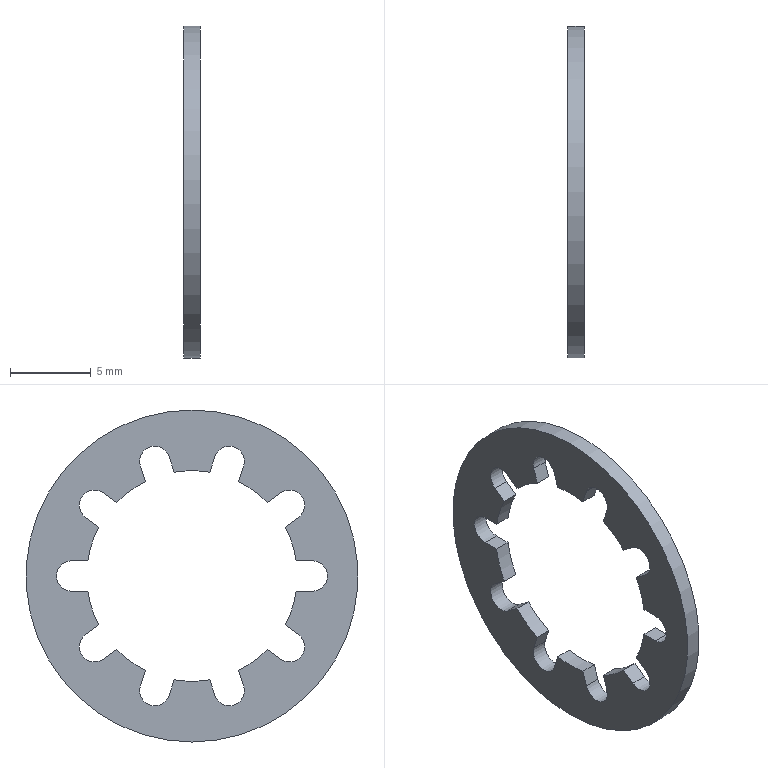Part | NX | features BREP 1 | 1 solid | 43 faces | box 1 x 20.5 x 20.5 mm | volume 165.523 mm3 | plane 22 | cylinder 21 | commonest cylinder face diameters 1.875 x10 13 x10 20.5 x1
STEP:
#1=CARTESIAN_POINT('',(0.,0.,10.25));
#2=VERTEX_POINT('',#1);
#3=CARTESIAN_POINT('',(0.,0.,0.));
#4=DIRECTION('',(1.,0.,0.));
#5=DIRECTION('',(0.,0.,1.));
#6=AXIS2_PLACEMENT_3D('',#3,#4,#5);
#7=CIRCLE('',#6,10.25);
#8=EDGE_CURVE('',#2,#2,#7,.T.);
#9=ORIENTED_EDGE('',*,*,#8,.F.);
#10=EDGE_LOOP('',(#9));
#11=FACE_BOUND('',#10,.T.);
#12=CARTESIAN_POINT('',(0.,3.19,6.784));
#13=VERTEX_POINT('',#12);
#14=CARTESIAN_POINT('',(0.,2.879,5.828));
#15=VERTEX_POINT('',#14);
#16=CARTESIAN_POINT('',(0.,3.19,6.784));
#17=DIRECTION('',(0.,-0.309,-0.9511));
#18=VECTOR('',#17,1000.);
#19=LINE('',#16,#18);
#20=EDGE_CURVE('',#13,#15,#19,.T.);
#21=ORIENTED_EDGE('',*,*,#20,.F.);
#22=CARTESIAN_POINT('',(0.,1.407,7.363));
#23=VERTEX_POINT('',#22);
#24=CARTESIAN_POINT('',(0.,2.298,7.073));
#25=DIRECTION('',(-1.,0.,0.));
#26=DIRECTION('',(0.,0.,1.));
#27=AXIS2_PLACEMENT_3D('',#24,#25,#26);
#28=CIRCLE('',#27,0.9375);
#29=EDGE_CURVE('',#23,#13,#28,.T.);
#30=ORIENTED_EDGE('',*,*,#29,.F.);
#31=CARTESIAN_POINT('',(0.,1.096,6.407));
#32=VERTEX_POINT('',#31);
#33=CARTESIAN_POINT('',(0.,1.096,6.407));
#34=DIRECTION('',(0.,0.309,0.9511));
#35=VECTOR('',#34,1000.);
#36=LINE('',#33,#35);
#37=EDGE_CURVE('',#32,#23,#36,.T.);
#38=ORIENTED_EDGE('',*,*,#37,.F.);
#39=CARTESIAN_POINT('',(0.,-1.096,6.407));
#40=VERTEX_POINT('',#39);
#41=CARTESIAN_POINT('',(0.,0.,0.));
#42=DIRECTION('',(-1.,0.,0.));
#43=DIRECTION('',(0.,0.,1.));
#44=AXIS2_PLACEMENT_3D('',#41,#42,#43);
#45=CIRCLE('',#44,6.5);
#46=EDGE_CURVE('',#40,#32,#45,.T.);
#47=ORIENTED_EDGE('',*,*,#46,.F.);
#48=CARTESIAN_POINT('',(0.,-1.407,7.363));
#49=VERTEX_POINT('',#48);
#50=CARTESIAN_POINT('',(0.,-1.407,7.363));
#51=DIRECTION('',(0.,0.309,-0.9511));
#52=VECTOR('',#51,1000.);
#53=LINE('',#50,#52);
#54=EDGE_CURVE('',#49,#40,#53,.T.);
#55=ORIENTED_EDGE('',*,*,#54,.F.);
#56=CARTESIAN_POINT('',(0.,-3.19,6.784));
#57=VERTEX_POINT('',#56);
#58=CARTESIAN_POINT('',(0.,-2.298,7.073));
#59=DIRECTION('',(-1.,0.,0.));
#60=DIRECTION('',(0.,0.,1.));
#61=AXIS2_PLACEMENT_3D('',#58,#59,#60);
#62=CIRCLE('',#61,0.9375);
#63=EDGE_CURVE('',#57,#49,#62,.T.);
#64=ORIENTED_EDGE('',*,*,#63,.F.);
#65=CARTESIAN_POINT('',(0.,-2.879,5.828));
#66=VERTEX_POINT('',#65);
#67=CARTESIAN_POINT('',(0.,-2.879,5.828));
#68=DIRECTION('',(0.,-0.309,0.9511));
#69=VECTOR('',#68,1000.);
#70=LINE('',#67,#69);
#71=EDGE_CURVE('',#66,#57,#70,.T.);
#72=ORIENTED_EDGE('',*,*,#71,.F.);
#73=CARTESIAN_POINT('',(0.,-4.653,4.539));
#74=VERTEX_POINT('',#73);
#75=CARTESIAN_POINT('',(0.,0.,0.));
#76=DIRECTION('',(-1.,0.,0.));
#77=DIRECTION('',(0.,0.,1.));
#78=AXIS2_PLACEMENT_3D('',#75,#76,#77);
#79=CIRCLE('',#78,6.5);
#80=EDGE_CURVE('',#74,#66,#79,.T.);
#81=ORIENTED_EDGE('',*,*,#80,.F.);
#82=CARTESIAN_POINT('',(0.,-5.466,5.13));
#83=VERTEX_POINT('',#82);
#84=CARTESIAN_POINT('',(0.,-5.466,5.13));
#85=DIRECTION('',(0.,0.809,-0.5878));
#86=VECTOR('',#85,1000.);
#87=LINE('',#84,#86);
#88=EDGE_CURVE('',#83,#74,#87,.T.);
#89=ORIENTED_EDGE('',*,*,#88,.F.);
#90=CARTESIAN_POINT('',(0.,-6.568,3.613));
#91=VERTEX_POINT('',#90);
#92=CARTESIAN_POINT('',(0.,-6.017,4.372));
#93=DIRECTION('',(-1.,0.,0.));
#94=DIRECTION('',(0.,0.,1.));
#95=AXIS2_PLACEMENT_3D('',#92,#93,#94);
#96=CIRCLE('',#95,0.9375);
#97=EDGE_CURVE('',#91,#83,#96,.T.);
#98=ORIENTED_EDGE('',*,*,#97,.F.);
#99=CARTESIAN_POINT('',(0.,-5.755,3.022));
#100=VERTEX_POINT('',#99);
#101=CARTESIAN_POINT('',(0.,-5.755,3.022));
#102=DIRECTION('',(0.,-0.809,0.5878));
#103=VECTOR('',#102,1000.);
#104=LINE('',#101,#103);
#105=EDGE_CURVE('',#100,#91,#104,.T.);
#106=ORIENTED_EDGE('',*,*,#105,.F.);
#107=CARTESIAN_POINT('',(0.,-6.432,0.9375));
#108=VERTEX_POINT('',#107);
#109=CARTESIAN_POINT('',(0.,0.,0.));
#110=DIRECTION('',(-1.,0.,0.));
#111=DIRECTION('',(0.,0.,1.));
#112=AXIS2_PLACEMENT_3D('',#109,#110,#111);
#113=CIRCLE('',#112,6.5);
#114=EDGE_CURVE('',#108,#100,#113,.T.);
#115=ORIENTED_EDGE('',*,*,#114,.F.);
#116=CARTESIAN_POINT('',(0.,-7.438,0.9375));
#117=VERTEX_POINT('',#116);
#118=CARTESIAN_POINT('',(0.,0.,0.9375));
#119=DIRECTION('',(0.,1.,0.));
#120=VECTOR('',#119,1000.);
#121=LINE('',#118,#120);
#122=EDGE_CURVE('',#117,#108,#121,.T.);
#123=ORIENTED_EDGE('',*,*,#122,.F.);
#124=CARTESIAN_POINT('',(0.,-7.438,-0.9375));
#125=VERTEX_POINT('',#124);
#126=CARTESIAN_POINT('',(0.,-7.438,0.));
#127=DIRECTION('',(-1.,0.,0.));
#128=DIRECTION('',(0.,0.,1.));
#129=AXIS2_PLACEMENT_3D('',#126,#127,#128);
#130=CIRCLE('',#129,0.9375);
#131=EDGE_CURVE('',#125,#117,#130,.T.);
#132=ORIENTED_EDGE('',*,*,#131,.F.);
#133=CARTESIAN_POINT('',(0.,-6.432,-0.9375));
#134=VERTEX_POINT('',#133);
#135=CARTESIAN_POINT('',(0.,0.,-0.9375));
#136=DIRECTION('',(0.,-1.,0.));
#137=VECTOR('',#136,1000.);
#138=LINE('',#135,#137);
#139=EDGE_CURVE('',#134,#125,#138,.T.);
#140=ORIENTED_EDGE('',*,*,#139,.F.);
#141=CARTESIAN_POINT('',(0.,-5.755,-3.022));
#142=VERTEX_POINT('',#141);
#143=CARTESIAN_POINT('',(0.,0.,0.));
#144=DIRECTION('',(-1.,0.,0.));
#145=DIRECTION('',(0.,0.,1.));
#146=AXIS2_PLACEMENT_3D('',#143,#144,#145);
#147=CIRCLE('',#146,6.5);
#148=EDGE_CURVE('',#142,#134,#147,.T.);
#149=ORIENTED_EDGE('',*,*,#148,.F.);
#150=CARTESIAN_POINT('',(0.,-6.568,-3.613));
#151=VERTEX_POINT('',#150);
#152=CARTESIAN_POINT('',(0.,-6.568,-3.613));
#153=DIRECTION('',(0.,0.809,0.5878));
#154=VECTOR('',#153,1000.);
#155=LINE('',#152,#154);
#156=EDGE_CURVE('',#151,#142,#155,.T.);
#157=ORIENTED_EDGE('',*,*,#156,.F.);
#158=CARTESIAN_POINT('',(0.,-5.466,-5.13));
#159=VERTEX_POINT('',#158);
#160=CARTESIAN_POINT('',(0.,-6.017,-4.372));
#161=DIRECTION('',(-1.,0.,0.));
#162=DIRECTION('',(0.,0.,1.));
#163=AXIS2_PLACEMENT_3D('',#160,#161,#162);
#164=CIRCLE('',#163,0.9375);
#165=EDGE_CURVE('',#159,#151,#164,.T.);
#166=ORIENTED_EDGE('',*,*,#165,.F.);
#167=CARTESIAN_POINT('',(0.,-4.653,-4.539));
#168=VERTEX_POINT('',#167);
#169=CARTESIAN_POINT('',(0.,-4.653,-4.539));
#170=DIRECTION('',(0.,-0.809,-0.5878));
#171=VECTOR('',#170,1000.);
#172=LINE('',#169,#171);
#173=EDGE_CURVE('',#168,#159,#172,.T.);
#174=ORIENTED_EDGE('',*,*,#173,.F.);
#175=CARTESIAN_POINT('',(0.,-2.879,-5.828));
#176=VERTEX_POINT('',#175);
#177=CARTESIAN_POINT('',(0.,0.,0.));
#178=DIRECTION('',(-1.,0.,0.));
#179=DIRECTION('',(0.,0.,1.));
#180=AXIS2_PLACEMENT_3D('',#177,#178,#179);
#181=CIRCLE('',#180,6.5);
#182=EDGE_CURVE('',#176,#168,#181,.T.);
#183=ORIENTED_EDGE('',*,*,#182,.F.);
#184=CARTESIAN_POINT('',(0.,-3.19,-6.784));
#185=VERTEX_POINT('',#184);
#186=CARTESIAN_POINT('',(0.,-3.19,-6.784));
#187=DIRECTION('',(0.,0.309,0.9511));
#188=VECTOR('',#187,1000.);
#189=LINE('',#186,#188);
#190=EDGE_CURVE('',#185,#176,#189,.T.);
#191=ORIENTED_EDGE('',*,*,#190,.F.);
#192=CARTESIAN_POINT('',(0.,-1.407,-7.363));
#193=VERTEX_POINT('',#192);
#194=CARTESIAN_POINT('',(0.,-2.298,-7.073));
#195=DIRECTION('',(-1.,0.,0.));
#196=DIRECTION('',(0.,0.,1.));
#197=AXIS2_PLACEMENT_3D('',#194,#195,#196);
#198=CIRCLE('',#197,0.9375);
#199=EDGE_CURVE('',#193,#185,#198,.T.);
#200=ORIENTED_EDGE('',*,*,#199,.F.);
#201=CARTESIAN_POINT('',(0.,-1.096,-6.407));
#202=VERTEX_POINT('',#201);
#203=CARTESIAN_POINT('',(0.,-1.096,-6.407));
#204=DIRECTION('',(0.,-0.309,-0.9511));
#205=VECTOR('',#204,1000.);
#206=LINE('',#203,#205);
#207=EDGE_CURVE('',#202,#193,#206,.T.);
#208=ORIENTED_EDGE('',*,*,#207,.F.);
#209=CARTESIAN_POINT('',(0.,1.096,-6.407));
#210=VERTEX_POINT('',#209);
#211=CARTESIAN_POINT('',(0.,0.,0.));
#212=DIRECTION('',(-1.,0.,0.));
#213=DIRECTION('',(0.,0.,1.));
#214=AXIS2_PLACEMENT_3D('',#211,#212,#213);
#215=CIRCLE('',#214,6.5);
#216=EDGE_CURVE('',#210,#202,#215,.T.);
#217=ORIENTED_EDGE('',*,*,#216,.F.);
#218=CARTESIAN_POINT('',(0.,1.407,-7.363));
#219=VERTEX_POINT('',#218);
#220=CARTESIAN_POINT('',(0.,1.407,-7.363));
#221=DIRECTION('',(0.,-0.309,0.9511));
#222=VECTOR('',#221,1000.);
#223=LINE('',#220,#222);
#224=EDGE_CURVE('',#219,#210,#223,.T.);
#225=ORIENTED_EDGE('',*,*,#224,.F.);
#226=CARTESIAN_POINT('',(0.,3.19,-6.784));
#227=VERTEX_POINT('',#226);
#228=CARTESIAN_POINT('',(0.,2.298,-7.073));
#229=DIRECTION('',(-1.,0.,0.));
#230=DIRECTION('',(0.,0.,1.));
#231=AXIS2_PLACEMENT_3D('',#228,#229,#230);
#232=CIRCLE('',#231,0.9375);
#233=EDGE_CURVE('',#227,#219,#232,.T.);
#234=ORIENTED_EDGE('',*,*,#233,.F.);
#235=CARTESIAN_POINT('',(0.,2.879,-5.828));
#236=VERTEX_POINT('',#235);
#237=CARTESIAN_POINT('',(0.,2.879,-5.828));
#238=DIRECTION('',(0.,0.309,-0.9511));
#239=VECTOR('',#238,1000.);
#240=LINE('',#237,#239);
#241=EDGE_CURVE('',#236,#227,#240,.T.);
#242=ORIENTED_EDGE('',*,*,#241,.F.);
#243=CARTESIAN_POINT('',(0.,4.653,-4.539));
#244=VERTEX_POINT('',#243);
#245=CARTESIAN_POINT('',(0.,0.,0.));
#246=DIRECTION('',(-1.,0.,0.));
#247=DIRECTION('',(0.,0.,1.));
#248=AXIS2_PLACEMENT_3D('',#245,#246,#247);
#249=CIRCLE('',#248,6.5);
#250=EDGE_CURVE('',#244,#236,#249,.T.);
#251=ORIENTED_EDGE('',*,*,#250,.F.);
#252=CARTESIAN_POINT('',(0.,5.466,-5.13));
#253=VERTEX_POINT('',#252);
#254=CARTESIAN_POINT('',(0.,5.466,-5.13));
#255=DIRECTION('',(0.,-0.809,0.5878));
#256=VECTOR('',#255,1000.);
#257=LINE('',#254,#256);
#258=EDGE_CURVE('',#253,#244,#257,.T.);
#259=ORIENTED_EDGE('',*,*,#258,.F.);
#260=CARTESIAN_POINT('',(0.,6.568,-3.613));
#261=VERTEX_POINT('',#260);
#262=CARTESIAN_POINT('',(0.,6.017,-4.372));
#263=DIRECTION('',(-1.,0.,0.));
#264=DIRECTION('',(0.,0.,1.));
#265=AXIS2_PLACEMENT_3D('',#262,#263,#264);
#266=CIRCLE('',#265,0.9375);
#267=EDGE_CURVE('',#261,#253,#266,.T.);
#268=ORIENTED_EDGE('',*,*,#267,.F.);
#269=CARTESIAN_POINT('',(0.,5.755,-3.022));
#270=VERTEX_POINT('',#269);
#271=CARTESIAN_POINT('',(0.,5.755,-3.022));
#272=DIRECTION('',(0.,0.809,-0.5878));
#273=VECTOR('',#272,1000.);
#274=LINE('',#271,#273);
#275=EDGE_CURVE('',#270,#261,#274,.T.);
#276=ORIENTED_EDGE('',*,*,#275,.F.);
#277=CARTESIAN_POINT('',(0.,6.432,-0.9375));
#278=VERTEX_POINT('',#277);
#279=CARTESIAN_POINT('',(0.,0.,0.));
#280=DIRECTION('',(-1.,0.,0.));
#281=DIRECTION('',(0.,0.,1.));
#282=AXIS2_PLACEMENT_3D('',#279,#280,#281);
#283=CIRCLE('',#282,6.5);
#284=EDGE_CURVE('',#278,#270,#283,.T.);
#285=ORIENTED_EDGE('',*,*,#284,.F.);
#286=CARTESIAN_POINT('',(0.,7.438,-0.9375));
#287=VERTEX_POINT('',#286);
#288=CARTESIAN_POINT('',(0.,0.,-0.9375));
#289=DIRECTION('',(0.,-1.,0.));
#290=VECTOR('',#289,1000.);
#291=LINE('',#288,#290);
#292=EDGE_CURVE('',#287,#278,#291,.T.);
#293=ORIENTED_EDGE('',*,*,#292,.F.);
#294=CARTESIAN_POINT('',(0.,7.438,0.9375));
#295=VERTEX_POINT('',#294);
#296=CARTESIAN_POINT('',(0.,7.438,0.));
#297=DIRECTION('',(-1.,0.,0.));
#298=DIRECTION('',(0.,0.,1.));
#299=AXIS2_PLACEMENT_3D('',#296,#297,#298);
#300=CIRCLE('',#299,0.9375);
#301=EDGE_CURVE('',#295,#287,#300,.T.);
#302=ORIENTED_EDGE('',*,*,#301,.F.);
#303=CARTESIAN_POINT('',(0.,6.432,0.9375));
#304=VERTEX_POINT('',#303);
#305=CARTESIAN_POINT('',(0.,0.,0.9375));
#306=DIRECTION('',(0.,1.,0.));
#307=VECTOR('',#306,1000.);
#308=LINE('',#305,#307);
#309=EDGE_CURVE('',#304,#295,#308,.T.);
#310=ORIENTED_EDGE('',*,*,#309,.F.);
#311=CARTESIAN_POINT('',(0.,5.755,3.022));
#312=VERTEX_POINT('',#311);
#313=CARTESIAN_POINT('',(0.,0.,0.));
#314=DIRECTION('',(-1.,0.,0.));
#315=DIRECTION('',(0.,0.,1.));
#316=AXIS2_PLACEMENT_3D('',#313,#314,#315);
#317=CIRCLE('',#316,6.5);
#318=EDGE_CURVE('',#312,#304,#317,.T.);
#319=ORIENTED_EDGE('',*,*,#318,.F.);
#320=CARTESIAN_POINT('',(0.,6.568,3.613));
#321=VERTEX_POINT('',#320);
#322=CARTESIAN_POINT('',(0.,6.568,3.613));
#323=DIRECTION('',(0.,-0.809,-0.5878));
#324=VECTOR('',#323,1000.);
#325=LINE('',#322,#324);
#326=EDGE_CURVE('',#321,#312,#325,.T.);
#327=ORIENTED_EDGE('',*,*,#326,.F.);
#328=CARTESIAN_POINT('',(0.,5.466,5.13));
#329=VERTEX_POINT('',#328);
#330=CARTESIAN_POINT('',(0.,6.017,4.372));
#331=DIRECTION('',(-1.,0.,0.));
#332=DIRECTION('',(0.,0.,1.));
#333=AXIS2_PLACEMENT_3D('',#330,#331,#332);
#334=CIRCLE('',#333,0.9375);
#335=EDGE_CURVE('',#329,#321,#334,.T.);
#336=ORIENTED_EDGE('',*,*,#335,.F.);
#337=CARTESIAN_POINT('',(0.,4.653,4.539));
#338=VERTEX_POINT('',#337);
#339=CARTESIAN_POINT('',(0.,4.653,4.539));
#340=DIRECTION('',(0.,0.809,0.5878));
#341=VECTOR('',#340,1000.);
#342=LINE('',#339,#341);
#343=EDGE_CURVE('',#338,#329,#342,.T.);
#344=ORIENTED_EDGE('',*,*,#343,.F.);
#345=CARTESIAN_POINT('',(0.,0.,0.));
#346=DIRECTION('',(-1.,0.,0.));
#347=DIRECTION('',(0.,0.,1.));
#348=AXIS2_PLACEMENT_3D('',#345,#346,#347);
#349=CIRCLE('',#348,6.5);
#350=EDGE_CURVE('',#15,#338,#349,.T.);
#351=ORIENTED_EDGE('',*,*,#350,.F.);
#352=EDGE_LOOP('',(#21,#30,#38,#47,#55,#64,#72,#81,#89,#98,#106,#115,#123,#132,#140,#149,#157,#166,#174,#183,#191,#200,#208,#217,#225,#234,#242,#251,#259,#268,#276,#285,#293,#302,#310,#319,#327,#336,#344,#351));
#353=FACE_BOUND('',#352,.T.);
#354=CARTESIAN_POINT('',(0.,0.,0.));
#355=DIRECTION('',(1.,0.,0.));
#356=DIRECTION('',(0.,0.,1.));
#357=AXIS2_PLACEMENT_3D('',#354,#355,#356);
#358=PLANE('',#357);
#359=ADVANCED_FACE('',(#11,#353),#358,.F.);
#360=CARTESIAN_POINT('',(1.,0.,10.25));
#361=VERTEX_POINT('',#360);
#362=CARTESIAN_POINT('',(1.,0.,0.));
#363=DIRECTION('',(-1.,0.,0.));
#364=DIRECTION('',(0.,0.,1.));
#365=AXIS2_PLACEMENT_3D('',#362,#363,#364);
#366=CIRCLE('',#365,10.25);
#367=EDGE_CURVE('',#361,#361,#366,.T.);
#368=ORIENTED_EDGE('',*,*,#367,.T.);
#369=EDGE_LOOP('',(#368));
#370=FACE_BOUND('',#369,.T.);
#371=ORIENTED_EDGE('',*,*,#8,.T.);
#372=EDGE_LOOP('',(#371));
#373=FACE_BOUND('',#372,.T.);
#374=CARTESIAN_POINT('',(1.,0.,0.));
#375=DIRECTION('',(-1.,0.,0.));
#376=DIRECTION('',(0.,0.,-1.));
#377=AXIS2_PLACEMENT_3D('',#374,#375,#376);
#378=CYLINDRICAL_SURFACE('',#377,10.25);
#379=ADVANCED_FACE('',(#370,#373),#378,.T.);
#380=CARTESIAN_POINT('',(1.,2.879,5.828));
#381=VERTEX_POINT('',#380);
#382=CARTESIAN_POINT('',(1.,3.19,6.784));
#383=VERTEX_POINT('',#382);
#384=CARTESIAN_POINT('',(1.,2.879,5.828));
#385=DIRECTION('',(0.,0.309,0.9511));
#386=VECTOR('',#385,1000.);
#387=LINE('',#384,#386);
#388=EDGE_CURVE('',#381,#383,#387,.T.);
#389=ORIENTED_EDGE('',*,*,#388,.T.);
#390=CARTESIAN_POINT('',(1.,3.19,6.784));
#391=DIRECTION('',(-1.,0.,0.));
#392=VECTOR('',#391,1000.);
#393=LINE('',#390,#392);
#394=EDGE_CURVE('',#383,#13,#393,.T.);
#395=ORIENTED_EDGE('',*,*,#394,.T.);
#396=ORIENTED_EDGE('',*,*,#20,.T.);
#397=CARTESIAN_POINT('',(1.,2.879,5.828));
#398=DIRECTION('',(1.,0.,0.));
#399=VECTOR('',#398,1000.);
#400=LINE('',#397,#399);
#401=EDGE_CURVE('',#15,#381,#400,.T.);
#402=ORIENTED_EDGE('',*,*,#401,.T.);
#403=EDGE_LOOP('',(#389,#395,#396,#402));
#404=FACE_BOUND('',#403,.T.);
#405=CARTESIAN_POINT('',(1.,2.879,5.828));
#406=DIRECTION('',(0.,-0.9511,0.309));
#407=DIRECTION('',(0.,0.309,0.9511));
#408=AXIS2_PLACEMENT_3D('',#405,#406,#407);
#409=PLANE('',#408);
#410=ADVANCED_FACE('',(#404),#409,.T.);
#411=CARTESIAN_POINT('',(1.,1.407,7.363));
#412=VERTEX_POINT('',#411);
#413=CARTESIAN_POINT('',(1.,2.298,7.073));
#414=DIRECTION('',(-1.,0.,0.));
#415=DIRECTION('',(0.,0.,1.));
#416=AXIS2_PLACEMENT_3D('',#413,#414,#415);
#417=CIRCLE('',#416,0.9375);
#418=EDGE_CURVE('',#412,#383,#417,.T.);
#419=ORIENTED_EDGE('',*,*,#418,.F.);
#420=CARTESIAN_POINT('',(1.,1.407,7.363));
#421=DIRECTION('',(1.,0.,0.));
#422=VECTOR('',#421,1000.);
#423=LINE('',#420,#422);
#424=EDGE_CURVE('',#23,#412,#423,.T.);
#425=ORIENTED_EDGE('',*,*,#424,.F.);
#426=ORIENTED_EDGE('',*,*,#29,.T.);
#427=ORIENTED_EDGE('',*,*,#394,.F.);
#428=EDGE_LOOP('',(#419,#425,#426,#427));
#429=FACE_BOUND('',#428,.T.);
#430=CARTESIAN_POINT('',(1.,2.298,7.073));
#431=DIRECTION('',(-1.,0.,0.));
#432=DIRECTION('',(0.,0.,-1.));
#433=AXIS2_PLACEMENT_3D('',#430,#431,#432);
#434=CYLINDRICAL_SURFACE('',#433,0.9375);
#435=ADVANCED_FACE('',(#429),#434,.F.);
#436=CARTESIAN_POINT('',(1.,1.096,6.407));
#437=VERTEX_POINT('',#436);
#438=CARTESIAN_POINT('',(1.,1.407,7.363));
#439=DIRECTION('',(0.,-0.309,-0.9511));
#440=VECTOR('',#439,1000.);
#441=LINE('',#438,#440);
#442=EDGE_CURVE('',#412,#437,#441,.T.);
#443=ORIENTED_EDGE('',*,*,#442,.T.);
#444=CARTESIAN_POINT('',(1.,1.096,6.407));
#445=DIRECTION('',(-1.,0.,0.));
#446=VECTOR('',#445,1000.);
#447=LINE('',#444,#446);
#448=EDGE_CURVE('',#437,#32,#447,.T.);
#449=ORIENTED_EDGE('',*,*,#448,.T.);
#450=ORIENTED_EDGE('',*,*,#37,.T.);
#451=ORIENTED_EDGE('',*,*,#424,.T.);
#452=EDGE_LOOP('',(#443,#449,#450,#451));
#453=FACE_BOUND('',#452,.T.);
#454=CARTESIAN_POINT('',(1.,1.407,7.363));
#455=DIRECTION('',(0.,0.9511,-0.309));
#456=DIRECTION('',(0.,-0.309,-0.9511));
#457=AXIS2_PLACEMENT_3D('',#454,#455,#456);
#458=PLANE('',#457);
#459=ADVANCED_FACE('',(#453),#458,.T.);
#460=CARTESIAN_POINT('',(1.,-1.096,6.407));
#461=VERTEX_POINT('',#460);
#462=CARTESIAN_POINT('',(1.,0.,0.));
#463=DIRECTION('',(-1.,0.,0.));
#464=DIRECTION('',(0.,0.,1.));
#465=AXIS2_PLACEMENT_3D('',#462,#463,#464);
#466=CIRCLE('',#465,6.5);
#467=EDGE_CURVE('',#461,#437,#466,.T.);
#468=ORIENTED_EDGE('',*,*,#467,.F.);
#469=CARTESIAN_POINT('',(1.,-1.096,6.407));
#470=DIRECTION('',(1.,0.,0.));
#471=VECTOR('',#470,1000.);
#472=LINE('',#469,#471);
#473=EDGE_CURVE('',#40,#461,#472,.T.);
#474=ORIENTED_EDGE('',*,*,#473,.F.);
#475=ORIENTED_EDGE('',*,*,#46,.T.);
#476=ORIENTED_EDGE('',*,*,#448,.F.);
#477=EDGE_LOOP('',(#468,#474,#475,#476));
#478=FACE_BOUND('',#477,.T.);
#479=CARTESIAN_POINT('',(1.,0.,0.));
#480=DIRECTION('',(-1.,0.,0.));
#481=DIRECTION('',(0.,0.,-1.));
#482=AXIS2_PLACEMENT_3D('',#479,#480,#481);
#483=CYLINDRICAL_SURFACE('',#482,6.5);
#484=ADVANCED_FACE('',(#478),#483,.F.);
#485=CARTESIAN_POINT('',(1.,-1.407,7.363));
#486=VERTEX_POINT('',#485);
#487=CARTESIAN_POINT('',(1.,-1.096,6.407));
#488=DIRECTION('',(0.,-0.309,0.9511));
#489=VECTOR('',#488,1000.);
#490=LINE('',#487,#489);
#491=EDGE_CURVE('',#461,#486,#490,.T.);
#492=ORIENTED_EDGE('',*,*,#491,.T.);
#493=CARTESIAN_POINT('',(1.,-1.407,7.363));
#494=DIRECTION('',(-1.,0.,0.));
#495=VECTOR('',#494,1000.);
#496=LINE('',#493,#495);
#497=EDGE_CURVE('',#486,#49,#496,.T.);
#498=ORIENTED_EDGE('',*,*,#497,.T.);
#499=ORIENTED_EDGE('',*,*,#54,.T.);
#500=ORIENTED_EDGE('',*,*,#473,.T.);
#501=EDGE_LOOP('',(#492,#498,#499,#500));
#502=FACE_BOUND('',#501,.T.);
#503=CARTESIAN_POINT('',(1.,-1.096,6.407));
#504=DIRECTION('',(0.,-0.9511,-0.309));
#505=DIRECTION('',(0.,-0.309,0.9511));
#506=AXIS2_PLACEMENT_3D('',#503,#504,#505);
#507=PLANE('',#506);
#508=ADVANCED_FACE('',(#502),#507,.T.);
#509=CARTESIAN_POINT('',(1.,-3.19,6.784));
#510=VERTEX_POINT('',#509);
#511=CARTESIAN_POINT('',(1.,-2.298,7.073));
#512=DIRECTION('',(-1.,0.,0.));
#513=DIRECTION('',(0.,0.,1.));
#514=AXIS2_PLACEMENT_3D('',#511,#512,#513);
#515=CIRCLE('',#514,0.9375);
#516=EDGE_CURVE('',#510,#486,#515,.T.);
#517=ORIENTED_EDGE('',*,*,#516,.F.);
#518=CARTESIAN_POINT('',(1.,-3.19,6.784));
#519=DIRECTION('',(1.,0.,0.));
#520=VECTOR('',#519,1000.);
#521=LINE('',#518,#520);
#522=EDGE_CURVE('',#57,#510,#521,.T.);
#523=ORIENTED_EDGE('',*,*,#522,.F.);
#524=ORIENTED_EDGE('',*,*,#63,.T.);
#525=ORIENTED_EDGE('',*,*,#497,.F.);
#526=EDGE_LOOP('',(#517,#523,#524,#525));
#527=FACE_BOUND('',#526,.T.);
#528=CARTESIAN_POINT('',(1.,-2.298,7.073));
#529=DIRECTION('',(-1.,0.,0.));
#530=DIRECTION('',(0.,0.,-1.));
#531=AXIS2_PLACEMENT_3D('',#528,#529,#530);
#532=CYLINDRICAL_SURFACE('',#531,0.9375);
#533=ADVANCED_FACE('',(#527),#532,.F.);
#534=CARTESIAN_POINT('',(1.,-2.879,5.828));
#535=VERTEX_POINT('',#534);
#536=CARTESIAN_POINT('',(1.,-3.19,6.784));
#537=DIRECTION('',(0.,0.309,-0.9511));
#538=VECTOR('',#537,1000.);
#539=LINE('',#536,#538);
#540=EDGE_CURVE('',#510,#535,#539,.T.);
#541=ORIENTED_EDGE('',*,*,#540,.T.);
#542=CARTESIAN_POINT('',(1.,-2.879,5.828));
#543=DIRECTION('',(-1.,0.,0.));
#544=VECTOR('',#543,1000.);
#545=LINE('',#542,#544);
#546=EDGE_CURVE('',#535,#66,#545,.T.);
#547=ORIENTED_EDGE('',*,*,#546,.T.);
#548=ORIENTED_EDGE('',*,*,#71,.T.);
#549=ORIENTED_EDGE('',*,*,#522,.T.);
#550=EDGE_LOOP('',(#541,#547,#548,#549));
#551=FACE_BOUND('',#550,.T.);
#552=CARTESIAN_POINT('',(1.,-3.19,6.784));
#553=DIRECTION('',(0.,0.9511,0.309));
#554=DIRECTION('',(0.,0.309,-0.9511));
#555=AXIS2_PLACEMENT_3D('',#552,#553,#554);
#556=PLANE('',#555);
#557=ADVANCED_FACE('',(#551),#556,.T.);
#558=ORIENTED_EDGE('',*,*,#546,.F.);
#559=CARTESIAN_POINT('',(1.,-4.653,4.539));
#560=VERTEX_POINT('',#559);
#561=CARTESIAN_POINT('',(1.,0.,0.));
#562=DIRECTION('',(-1.,0.,0.));
#563=DIRECTION('',(0.,0.,1.));
#564=AXIS2_PLACEMENT_3D('',#561,#562,#563);
#565=CIRCLE('',#564,6.5);
#566=EDGE_CURVE('',#560,#535,#565,.T.);
#567=ORIENTED_EDGE('',*,*,#566,.F.);
#568=CARTESIAN_POINT('',(1.,-4.653,4.539));
#569=DIRECTION('',(1.,0.,0.));
#570=VECTOR('',#569,1000.);
#571=LINE('',#568,#570);
#572=EDGE_CURVE('',#74,#560,#571,.T.);
#573=ORIENTED_EDGE('',*,*,#572,.F.);
#574=ORIENTED_EDGE('',*,*,#80,.T.);
#575=EDGE_LOOP('',(#558,#567,#573,#574));
#576=FACE_BOUND('',#575,.T.);
#577=CARTESIAN_POINT('',(1.,0.,0.));
#578=DIRECTION('',(-1.,0.,0.));
#579=DIRECTION('',(0.,0.,-1.));
#580=AXIS2_PLACEMENT_3D('',#577,#578,#579);
#581=CYLINDRICAL_SURFACE('',#580,6.5);
#582=ADVANCED_FACE('',(#576),#581,.F.);
#583=CARTESIAN_POINT('',(1.,-5.466,5.13));
#584=VERTEX_POINT('',#583);
#585=CARTESIAN_POINT('',(1.,-4.653,4.539));
#586=DIRECTION('',(0.,-0.809,0.5878));
#587=VECTOR('',#586,1000.);
#588=LINE('',#585,#587);
#589=EDGE_CURVE('',#560,#584,#588,.T.);
#590=ORIENTED_EDGE('',*,*,#589,.T.);
#591=CARTESIAN_POINT('',(1.,-5.466,5.13));
#592=DIRECTION('',(-1.,0.,0.));
#593=VECTOR('',#592,1000.);
#594=LINE('',#591,#593);
#595=EDGE_CURVE('',#584,#83,#594,.T.);
#596=ORIENTED_EDGE('',*,*,#595,.T.);
#597=ORIENTED_EDGE('',*,*,#88,.T.);
#598=ORIENTED_EDGE('',*,*,#572,.T.);
#599=EDGE_LOOP('',(#590,#596,#597,#598));
#600=FACE_BOUND('',#599,.T.);
#601=CARTESIAN_POINT('',(1.,-4.653,4.539));
#602=DIRECTION('',(0.,-0.5878,-0.809));
#603=DIRECTION('',(0.,-0.809,0.5878));
#604=AXIS2_PLACEMENT_3D('',#601,#602,#603);
#605=PLANE('',#604);
#606=ADVANCED_FACE('',(#600),#605,.T.);
#607=CARTESIAN_POINT('',(1.,-6.568,3.613));
#608=VERTEX_POINT('',#607);
#609=CARTESIAN_POINT('',(1.,-6.017,4.372));
#610=DIRECTION('',(-1.,0.,0.));
#611=DIRECTION('',(0.,0.,1.));
#612=AXIS2_PLACEMENT_3D('',#609,#610,#611);
#613=CIRCLE('',#612,0.9375);
#614=EDGE_CURVE('',#608,#584,#613,.T.);
#615=ORIENTED_EDGE('',*,*,#614,.F.);
#616=CARTESIAN_POINT('',(1.,-6.568,3.613));
#617=DIRECTION('',(1.,0.,0.));
#618=VECTOR('',#617,1000.);
#619=LINE('',#616,#618);
#620=EDGE_CURVE('',#91,#608,#619,.T.);
#621=ORIENTED_EDGE('',*,*,#620,.F.);
#622=ORIENTED_EDGE('',*,*,#97,.T.);
#623=ORIENTED_EDGE('',*,*,#595,.F.);
#624=EDGE_LOOP('',(#615,#621,#622,#623));
#625=FACE_BOUND('',#624,.T.);
#626=CARTESIAN_POINT('',(1.,-6.017,4.372));
#627=DIRECTION('',(-1.,0.,0.));
#628=DIRECTION('',(0.,0.,-1.));
#629=AXIS2_PLACEMENT_3D('',#626,#627,#628);
#630=CYLINDRICAL_SURFACE('',#629,0.9375);
#631=ADVANCED_FACE('',(#625),#630,.F.);
#632=CARTESIAN_POINT('',(1.,-5.755,3.022));
#633=VERTEX_POINT('',#632);
#634=CARTESIAN_POINT('',(1.,-6.568,3.613));
#635=DIRECTION('',(0.,0.809,-0.5878));
#636=VECTOR('',#635,1000.);
#637=LINE('',#634,#636);
#638=EDGE_CURVE('',#608,#633,#637,.T.);
#639=ORIENTED_EDGE('',*,*,#638,.T.);
#640=CARTESIAN_POINT('',(1.,-5.755,3.022));
#641=DIRECTION('',(-1.,0.,0.));
#642=VECTOR('',#641,1000.);
#643=LINE('',#640,#642);
#644=EDGE_CURVE('',#633,#100,#643,.T.);
#645=ORIENTED_EDGE('',*,*,#644,.T.);
#646=ORIENTED_EDGE('',*,*,#105,.T.);
#647=ORIENTED_EDGE('',*,*,#620,.T.);
#648=EDGE_LOOP('',(#639,#645,#646,#647));
#649=FACE_BOUND('',#648,.T.);
#650=CARTESIAN_POINT('',(1.,-6.568,3.613));
#651=DIRECTION('',(0.,0.5878,0.809));
#652=DIRECTION('',(0.,0.809,-0.5878));
#653=AXIS2_PLACEMENT_3D('',#650,#651,#652);
#654=PLANE('',#653);
#655=ADVANCED_FACE('',(#649),#654,.T.);
#656=ORIENTED_EDGE('',*,*,#644,.F.);
#657=CARTESIAN_POINT('',(1.,-6.432,0.9375));
#658=VERTEX_POINT('',#657);
#659=CARTESIAN_POINT('',(1.,0.,0.));
#660=DIRECTION('',(-1.,0.,0.));
#661=DIRECTION('',(0.,0.,1.));
#662=AXIS2_PLACEMENT_3D('',#659,#660,#661);
#663=CIRCLE('',#662,6.5);
#664=EDGE_CURVE('',#658,#633,#663,.T.);
#665=ORIENTED_EDGE('',*,*,#664,.F.);
#666=CARTESIAN_POINT('',(1.,-6.432,0.9375));
#667=DIRECTION('',(1.,0.,0.));
#668=VECTOR('',#667,1000.);
#669=LINE('',#666,#668);
#670=EDGE_CURVE('',#108,#658,#669,.T.);
#671=ORIENTED_EDGE('',*,*,#670,.F.);
#672=ORIENTED_EDGE('',*,*,#114,.T.);
#673=EDGE_LOOP('',(#656,#665,#671,#672));
#674=FACE_BOUND('',#673,.T.);
#675=CARTESIAN_POINT('',(1.,0.,0.));
#676=DIRECTION('',(-1.,0.,0.));
#677=DIRECTION('',(0.,0.,-1.));
#678=AXIS2_PLACEMENT_3D('',#675,#676,#677);
#679=CYLINDRICAL_SURFACE('',#678,6.5);
#680=ADVANCED_FACE('',(#674),#679,.F.);
#681=CARTESIAN_POINT('',(1.,-7.438,0.9375));
#682=VERTEX_POINT('',#681);
#683=CARTESIAN_POINT('',(1.,-6.432,0.9375));
#684=DIRECTION('',(0.,-1.,0.));
#685=VECTOR('',#684,1000.);
#686=LINE('',#683,#685);
#687=EDGE_CURVE('',#658,#682,#686,.T.);
#688=ORIENTED_EDGE('',*,*,#687,.T.);
#689=CARTESIAN_POINT('',(1.,-7.438,0.9375));
#690=DIRECTION('',(-1.,0.,0.));
#691=VECTOR('',#690,1000.);
#692=LINE('',#689,#691);
#693=EDGE_CURVE('',#682,#117,#692,.T.);
#694=ORIENTED_EDGE('',*,*,#693,.T.);
#695=ORIENTED_EDGE('',*,*,#122,.T.);
#696=ORIENTED_EDGE('',*,*,#670,.T.);
#697=EDGE_LOOP('',(#688,#694,#695,#696));
#698=FACE_BOUND('',#697,.T.);
#699=CARTESIAN_POINT('',(1.,-6.432,0.9375));
#700=DIRECTION('',(0.,0.,-1.));
#701=DIRECTION('',(1.,0.,0.));
#702=AXIS2_PLACEMENT_3D('',#699,#700,#701);
#703=PLANE('',#702);
#704=ADVANCED_FACE('',(#698),#703,.T.);
#705=ORIENTED_EDGE('',*,*,#693,.F.);
#706=CARTESIAN_POINT('',(1.,-7.438,-0.9375));
#707=VERTEX_POINT('',#706);
#708=CARTESIAN_POINT('',(1.,-7.438,0.));
#709=DIRECTION('',(-1.,0.,0.));
#710=DIRECTION('',(0.,0.,1.));
#711=AXIS2_PLACEMENT_3D('',#708,#709,#710);
#712=CIRCLE('',#711,0.9375);
#713=EDGE_CURVE('',#707,#682,#712,.T.);
#714=ORIENTED_EDGE('',*,*,#713,.F.);
#715=CARTESIAN_POINT('',(1.,-7.438,-0.9375));
#716=DIRECTION('',(1.,0.,0.));
#717=VECTOR('',#716,1000.);
#718=LINE('',#715,#717);
#719=EDGE_CURVE('',#125,#707,#718,.T.);
#720=ORIENTED_EDGE('',*,*,#719,.F.);
#721=ORIENTED_EDGE('',*,*,#131,.T.);
#722=EDGE_LOOP('',(#705,#714,#720,#721));
#723=FACE_BOUND('',#722,.T.);
#724=CARTESIAN_POINT('',(1.,-7.438,0.));
#725=DIRECTION('',(-1.,0.,0.));
#726=DIRECTION('',(0.,0.,-1.));
#727=AXIS2_PLACEMENT_3D('',#724,#725,#726);
#728=CYLINDRICAL_SURFACE('',#727,0.9375);
#729=ADVANCED_FACE('',(#723),#728,.F.);
#730=CARTESIAN_POINT('',(1.,-6.432,-0.9375));
#731=VERTEX_POINT('',#730);
#732=CARTESIAN_POINT('',(1.,-7.438,-0.9375));
#733=DIRECTION('',(0.,1.,0.));
#734=VECTOR('',#733,1000.);
#735=LINE('',#732,#734);
#736=EDGE_CURVE('',#707,#731,#735,.T.);
#737=ORIENTED_EDGE('',*,*,#736,.T.);
#738=CARTESIAN_POINT('',(1.,-6.432,-0.9375));
#739=DIRECTION('',(-1.,0.,0.));
#740=VECTOR('',#739,1000.);
#741=LINE('',#738,#740);
#742=EDGE_CURVE('',#731,#134,#741,.T.);
#743=ORIENTED_EDGE('',*,*,#742,.T.);
#744=ORIENTED_EDGE('',*,*,#139,.T.);
#745=ORIENTED_EDGE('',*,*,#719,.T.);
#746=EDGE_LOOP('',(#737,#743,#744,#745));
#747=FACE_BOUND('',#746,.T.);
#748=CARTESIAN_POINT('',(1.,-7.438,-0.9375));
#749=DIRECTION('',(0.,0.,1.));
#750=DIRECTION('',(0.,1.,0.));
#751=AXIS2_PLACEMENT_3D('',#748,#749,#750);
#752=PLANE('',#751);
#753=ADVANCED_FACE('',(#747),#752,.T.);
#754=ORIENTED_EDGE('',*,*,#742,.F.);
#755=CARTESIAN_POINT('',(1.,-5.755,-3.022));
#756=VERTEX_POINT('',#755);
#757=CARTESIAN_POINT('',(1.,0.,0.));
#758=DIRECTION('',(-1.,0.,0.));
#759=DIRECTION('',(0.,0.,1.));
#760=AXIS2_PLACEMENT_3D('',#757,#758,#759);
#761=CIRCLE('',#760,6.5);
#762=EDGE_CURVE('',#756,#731,#761,.T.);
#763=ORIENTED_EDGE('',*,*,#762,.F.);
#764=CARTESIAN_POINT('',(1.,-5.755,-3.022));
#765=DIRECTION('',(1.,0.,0.));
#766=VECTOR('',#765,1000.);
#767=LINE('',#764,#766);
#768=EDGE_CURVE('',#142,#756,#767,.T.);
#769=ORIENTED_EDGE('',*,*,#768,.F.);
#770=ORIENTED_EDGE('',*,*,#148,.T.);
#771=EDGE_LOOP('',(#754,#763,#769,#770));
#772=FACE_BOUND('',#771,.T.);
#773=CARTESIAN_POINT('',(1.,0.,0.));
#774=DIRECTION('',(-1.,0.,0.));
#775=DIRECTION('',(0.,0.,-1.));
#776=AXIS2_PLACEMENT_3D('',#773,#774,#775);
#777=CYLINDRICAL_SURFACE('',#776,6.5);
#778=ADVANCED_FACE('',(#772),#777,.F.);
#779=CARTESIAN_POINT('',(1.,-6.568,-3.613));
#780=VERTEX_POINT('',#779);
#781=CARTESIAN_POINT('',(1.,-5.755,-3.022));
#782=DIRECTION('',(0.,-0.809,-0.5878));
#783=VECTOR('',#782,1000.);
#784=LINE('',#781,#783);
#785=EDGE_CURVE('',#756,#780,#784,.T.);
#786=ORIENTED_EDGE('',*,*,#785,.T.);
#787=CARTESIAN_POINT('',(1.,-6.568,-3.613));
#788=DIRECTION('',(-1.,0.,0.));
#789=VECTOR('',#788,1000.);
#790=LINE('',#787,#789);
#791=EDGE_CURVE('',#780,#151,#790,.T.);
#792=ORIENTED_EDGE('',*,*,#791,.T.);
#793=ORIENTED_EDGE('',*,*,#156,.T.);
#794=ORIENTED_EDGE('',*,*,#768,.T.);
#795=EDGE_LOOP('',(#786,#792,#793,#794));
#796=FACE_BOUND('',#795,.T.);
#797=CARTESIAN_POINT('',(1.,-5.755,-3.022));
#798=DIRECTION('',(0.,0.5878,-0.809));
#799=DIRECTION('',(0.,-0.809,-0.5878));
#800=AXIS2_PLACEMENT_3D('',#797,#798,#799);
#801=PLANE('',#800);
#802=ADVANCED_FACE('',(#796),#801,.T.);
#803=ORIENTED_EDGE('',*,*,#791,.F.);
#804=CARTESIAN_POINT('',(1.,-5.466,-5.13));
#805=VERTEX_POINT('',#804);
#806=CARTESIAN_POINT('',(1.,-6.017,-4.372));
#807=DIRECTION('',(-1.,0.,0.));
#808=DIRECTION('',(0.,0.,1.));
#809=AXIS2_PLACEMENT_3D('',#806,#807,#808);
#810=CIRCLE('',#809,0.9375);
#811=EDGE_CURVE('',#805,#780,#810,.T.);
#812=ORIENTED_EDGE('',*,*,#811,.F.);
#813=CARTESIAN_POINT('',(1.,-5.466,-5.13));
#814=DIRECTION('',(1.,0.,0.));
#815=VECTOR('',#814,1000.);
#816=LINE('',#813,#815);
#817=EDGE_CURVE('',#159,#805,#816,.T.);
#818=ORIENTED_EDGE('',*,*,#817,.F.);
#819=ORIENTED_EDGE('',*,*,#165,.T.);
#820=EDGE_LOOP('',(#803,#812,#818,#819));
#821=FACE_BOUND('',#820,.T.);
#822=CARTESIAN_POINT('',(1.,-6.017,-4.372));
#823=DIRECTION('',(-1.,0.,0.));
#824=DIRECTION('',(0.,0.,-1.));
#825=AXIS2_PLACEMENT_3D('',#822,#823,#824);
#826=CYLINDRICAL_SURFACE('',#825,0.9375);
#827=ADVANCED_FACE('',(#821),#826,.F.);
#828=CARTESIAN_POINT('',(1.,-4.653,-4.539));
#829=VERTEX_POINT('',#828);
#830=CARTESIAN_POINT('',(1.,-5.466,-5.13));
#831=DIRECTION('',(0.,0.809,0.5878));
#832=VECTOR('',#831,1000.);
#833=LINE('',#830,#832);
#834=EDGE_CURVE('',#805,#829,#833,.T.);
#835=ORIENTED_EDGE('',*,*,#834,.T.);
#836=CARTESIAN_POINT('',(1.,-4.653,-4.539));
#837=DIRECTION('',(-1.,0.,0.));
#838=VECTOR('',#837,1000.);
#839=LINE('',#836,#838);
#840=EDGE_CURVE('',#829,#168,#839,.T.);
#841=ORIENTED_EDGE('',*,*,#840,.T.);
#842=ORIENTED_EDGE('',*,*,#173,.T.);
#843=ORIENTED_EDGE('',*,*,#817,.T.);
#844=EDGE_LOOP('',(#835,#841,#842,#843));
#845=FACE_BOUND('',#844,.T.);
#846=CARTESIAN_POINT('',(1.,-5.466,-5.13));
#847=DIRECTION('',(0.,-0.5878,0.809));
#848=DIRECTION('',(0.,0.809,0.5878));
#849=AXIS2_PLACEMENT_3D('',#846,#847,#848);
#850=PLANE('',#849);
#851=ADVANCED_FACE('',(#845),#850,.T.);
#852=ORIENTED_EDGE('',*,*,#840,.F.);
#853=CARTESIAN_POINT('',(1.,-2.879,-5.828));
#854=VERTEX_POINT('',#853);
#855=CARTESIAN_POINT('',(1.,0.,0.));
#856=DIRECTION('',(-1.,0.,0.));
#857=DIRECTION('',(0.,0.,1.));
#858=AXIS2_PLACEMENT_3D('',#855,#856,#857);
#859=CIRCLE('',#858,6.5);
#860=EDGE_CURVE('',#854,#829,#859,.T.);
#861=ORIENTED_EDGE('',*,*,#860,.F.);
#862=CARTESIAN_POINT('',(1.,-2.879,-5.828));
#863=DIRECTION('',(1.,0.,0.));
#864=VECTOR('',#863,1000.);
#865=LINE('',#862,#864);
#866=EDGE_CURVE('',#176,#854,#865,.T.);
#867=ORIENTED_EDGE('',*,*,#866,.F.);
#868=ORIENTED_EDGE('',*,*,#182,.T.);
#869=EDGE_LOOP('',(#852,#861,#867,#868));
#870=FACE_BOUND('',#869,.T.);
#871=CARTESIAN_POINT('',(1.,0.,0.));
#872=DIRECTION('',(-1.,0.,0.));
#873=DIRECTION('',(0.,0.,-1.));
#874=AXIS2_PLACEMENT_3D('',#871,#872,#873);
#875=CYLINDRICAL_SURFACE('',#874,6.5);
#876=ADVANCED_FACE('',(#870),#875,.F.);
#877=CARTESIAN_POINT('',(1.,-3.19,-6.784));
#878=VERTEX_POINT('',#877);
#879=CARTESIAN_POINT('',(1.,-2.879,-5.828));
#880=DIRECTION('',(0.,-0.309,-0.9511));
#881=VECTOR('',#880,1000.);
#882=LINE('',#879,#881);
#883=EDGE_CURVE('',#854,#878,#882,.T.);
#884=ORIENTED_EDGE('',*,*,#883,.T.);
#885=CARTESIAN_POINT('',(1.,-3.19,-6.784));
#886=DIRECTION('',(-1.,0.,0.));
#887=VECTOR('',#886,1000.);
#888=LINE('',#885,#887);
#889=EDGE_CURVE('',#878,#185,#888,.T.);
#890=ORIENTED_EDGE('',*,*,#889,.T.);
#891=ORIENTED_EDGE('',*,*,#190,.T.);
#892=ORIENTED_EDGE('',*,*,#866,.T.);
#893=EDGE_LOOP('',(#884,#890,#891,#892));
#894=FACE_BOUND('',#893,.T.);
#895=CARTESIAN_POINT('',(1.,-2.879,-5.828));
#896=DIRECTION('',(0.,0.9511,-0.309));
#897=DIRECTION('',(0.,-0.309,-0.9511));
#898=AXIS2_PLACEMENT_3D('',#895,#896,#897);
#899=PLANE('',#898);
#900=ADVANCED_FACE('',(#894),#899,.T.);
#901=ORIENTED_EDGE('',*,*,#889,.F.);
#902=CARTESIAN_POINT('',(1.,-1.407,-7.363));
#903=VERTEX_POINT('',#902);
#904=CARTESIAN_POINT('',(1.,-2.298,-7.073));
#905=DIRECTION('',(-1.,0.,0.));
#906=DIRECTION('',(0.,0.,1.));
#907=AXIS2_PLACEMENT_3D('',#904,#905,#906);
#908=CIRCLE('',#907,0.9375);
#909=EDGE_CURVE('',#903,#878,#908,.T.);
#910=ORIENTED_EDGE('',*,*,#909,.F.);
#911=CARTESIAN_POINT('',(1.,-1.407,-7.363));
#912=DIRECTION('',(1.,0.,0.));
#913=VECTOR('',#912,1000.);
#914=LINE('',#911,#913);
#915=EDGE_CURVE('',#193,#903,#914,.T.);
#916=ORIENTED_EDGE('',*,*,#915,.F.);
#917=ORIENTED_EDGE('',*,*,#199,.T.);
#918=EDGE_LOOP('',(#901,#910,#916,#917));
#919=FACE_BOUND('',#918,.T.);
#920=CARTESIAN_POINT('',(1.,-2.298,-7.073));
#921=DIRECTION('',(-1.,0.,0.));
#922=DIRECTION('',(0.,0.,-1.));
#923=AXIS2_PLACEMENT_3D('',#920,#921,#922);
#924=CYLINDRICAL_SURFACE('',#923,0.9375);
#925=ADVANCED_FACE('',(#919),#924,.F.);
#926=CARTESIAN_POINT('',(1.,-1.096,-6.407));
#927=VERTEX_POINT('',#926);
#928=CARTESIAN_POINT('',(1.,-1.407,-7.363));
#929=DIRECTION('',(0.,0.309,0.9511));
#930=VECTOR('',#929,1000.);
#931=LINE('',#928,#930);
#932=EDGE_CURVE('',#903,#927,#931,.T.);
#933=ORIENTED_EDGE('',*,*,#932,.T.);
#934=CARTESIAN_POINT('',(1.,-1.096,-6.407));
#935=DIRECTION('',(-1.,0.,0.));
#936=VECTOR('',#935,1000.);
#937=LINE('',#934,#936);
#938=EDGE_CURVE('',#927,#202,#937,.T.);
#939=ORIENTED_EDGE('',*,*,#938,.T.);
#940=ORIENTED_EDGE('',*,*,#207,.T.);
#941=ORIENTED_EDGE('',*,*,#915,.T.);
#942=EDGE_LOOP('',(#933,#939,#940,#941));
#943=FACE_BOUND('',#942,.T.);
#944=CARTESIAN_POINT('',(1.,-1.407,-7.363));
#945=DIRECTION('',(0.,-0.9511,0.309));
#946=DIRECTION('',(0.,0.309,0.9511));
#947=AXIS2_PLACEMENT_3D('',#944,#945,#946);
#948=PLANE('',#947);
#949=ADVANCED_FACE('',(#943),#948,.T.);
#950=ORIENTED_EDGE('',*,*,#938,.F.);
#951=CARTESIAN_POINT('',(1.,1.096,-6.407));
#952=VERTEX_POINT('',#951);
#953=CARTESIAN_POINT('',(1.,0.,0.));
#954=DIRECTION('',(-1.,0.,0.));
#955=DIRECTION('',(0.,0.,1.));
#956=AXIS2_PLACEMENT_3D('',#953,#954,#955);
#957=CIRCLE('',#956,6.5);
#958=EDGE_CURVE('',#952,#927,#957,.T.);
#959=ORIENTED_EDGE('',*,*,#958,.F.);
#960=CARTESIAN_POINT('',(1.,1.096,-6.407));
#961=DIRECTION('',(1.,0.,0.));
#962=VECTOR('',#961,1000.);
#963=LINE('',#960,#962);
#964=EDGE_CURVE('',#210,#952,#963,.T.);
#965=ORIENTED_EDGE('',*,*,#964,.F.);
#966=ORIENTED_EDGE('',*,*,#216,.T.);
#967=EDGE_LOOP('',(#950,#959,#965,#966));
#968=FACE_BOUND('',#967,.T.);
#969=CARTESIAN_POINT('',(1.,0.,0.));
#970=DIRECTION('',(-1.,0.,0.));
#971=DIRECTION('',(0.,0.,-1.));
#972=AXIS2_PLACEMENT_3D('',#969,#970,#971);
#973=CYLINDRICAL_SURFACE('',#972,6.5);
#974=ADVANCED_FACE('',(#968),#973,.F.);
#975=CARTESIAN_POINT('',(1.,1.407,-7.363));
#976=VERTEX_POINT('',#975);
#977=CARTESIAN_POINT('',(1.,1.096,-6.407));
#978=DIRECTION('',(0.,0.309,-0.9511));
#979=VECTOR('',#978,1000.);
#980=LINE('',#977,#979);
#981=EDGE_CURVE('',#952,#976,#980,.T.);
#982=ORIENTED_EDGE('',*,*,#981,.T.);
#983=CARTESIAN_POINT('',(1.,1.407,-7.363));
#984=DIRECTION('',(-1.,0.,0.));
#985=VECTOR('',#984,1000.);
#986=LINE('',#983,#985);
#987=EDGE_CURVE('',#976,#219,#986,.T.);
#988=ORIENTED_EDGE('',*,*,#987,.T.);
#989=ORIENTED_EDGE('',*,*,#224,.T.);
#990=ORIENTED_EDGE('',*,*,#964,.T.);
#991=EDGE_LOOP('',(#982,#988,#989,#990));
#992=FACE_BOUND('',#991,.T.);
#993=CARTESIAN_POINT('',(1.,1.096,-6.407));
#994=DIRECTION('',(0.,0.9511,0.309));
#995=DIRECTION('',(0.,0.309,-0.9511));
#996=AXIS2_PLACEMENT_3D('',#993,#994,#995);
#997=PLANE('',#996);
#998=ADVANCED_FACE('',(#992),#997,.T.);
#999=ORIENTED_EDGE('',*,*,#987,.F.);
#1000=CARTESIAN_POINT('',(1.,3.19,-6.784));
#1001=VERTEX_POINT('',#1000);
#1002=CARTESIAN_POINT('',(1.,2.298,-7.073));
#1003=DIRECTION('',(-1.,0.,0.));
#1004=DIRECTION('',(0.,0.,1.));
#1005=AXIS2_PLACEMENT_3D('',#1002,#1003,#1004);
#1006=CIRCLE('',#1005,0.9375);
#1007=EDGE_CURVE('',#1001,#976,#1006,.T.);
#1008=ORIENTED_EDGE('',*,*,#1007,.F.);
#1009=CARTESIAN_POINT('',(1.,3.19,-6.784));
#1010=DIRECTION('',(1.,0.,0.));
#1011=VECTOR('',#1010,1000.);
#1012=LINE('',#1009,#1011);
#1013=EDGE_CURVE('',#227,#1001,#1012,.T.);
#1014=ORIENTED_EDGE('',*,*,#1013,.F.);
#1015=ORIENTED_EDGE('',*,*,#233,.T.);
#1016=EDGE_LOOP('',(#999,#1008,#1014,#1015));
#1017=FACE_BOUND('',#1016,.T.);
#1018=CARTESIAN_POINT('',(1.,2.298,-7.073));
#1019=DIRECTION('',(-1.,0.,0.));
#1020=DIRECTION('',(0.,0.,-1.));
#1021=AXIS2_PLACEMENT_3D('',#1018,#1019,#1020);
#1022=CYLINDRICAL_SURFACE('',#1021,0.9375);
#1023=ADVANCED_FACE('',(#1017),#1022,.F.);
#1024=CARTESIAN_POINT('',(1.,2.879,-5.828));
#1025=VERTEX_POINT('',#1024);
#1026=CARTESIAN_POINT('',(1.,3.19,-6.784));
#1027=DIRECTION('',(0.,-0.309,0.9511));
#1028=VECTOR('',#1027,1000.);
#1029=LINE('',#1026,#1028);
#1030=EDGE_CURVE('',#1001,#1025,#1029,.T.);
#1031=ORIENTED_EDGE('',*,*,#1030,.T.);
#1032=CARTESIAN_POINT('',(1.,2.879,-5.828));
#1033=DIRECTION('',(-1.,0.,0.));
#1034=VECTOR('',#1033,1000.);
#1035=LINE('',#1032,#1034);
#1036=EDGE_CURVE('',#1025,#236,#1035,.T.);
#1037=ORIENTED_EDGE('',*,*,#1036,.T.);
#1038=ORIENTED_EDGE('',*,*,#241,.T.);
#1039=ORIENTED_EDGE('',*,*,#1013,.T.);
#1040=EDGE_LOOP('',(#1031,#1037,#1038,#1039));
#1041=FACE_BOUND('',#1040,.T.);
#1042=CARTESIAN_POINT('',(1.,3.19,-6.784));
#1043=DIRECTION('',(0.,-0.9511,-0.309));
#1044=DIRECTION('',(0.,-0.309,0.9511));
#1045=AXIS2_PLACEMENT_3D('',#1042,#1043,#1044);
#1046=PLANE('',#1045);
#1047=ADVANCED_FACE('',(#1041),#1046,.T.);
#1048=ORIENTED_EDGE('',*,*,#1036,.F.);
#1049=CARTESIAN_POINT('',(1.,4.653,-4.539));
#1050=VERTEX_POINT('',#1049);
#1051=CARTESIAN_POINT('',(1.,0.,0.));
#1052=DIRECTION('',(-1.,0.,0.));
#1053=DIRECTION('',(0.,0.,1.));
#1054=AXIS2_PLACEMENT_3D('',#1051,#1052,#1053);
#1055=CIRCLE('',#1054,6.5);
#1056=EDGE_CURVE('',#1050,#1025,#1055,.T.);
#1057=ORIENTED_EDGE('',*,*,#1056,.F.);
#1058=CARTESIAN_POINT('',(1.,4.653,-4.539));
#1059=DIRECTION('',(1.,0.,0.));
#1060=VECTOR('',#1059,1000.);
#1061=LINE('',#1058,#1060);
#1062=EDGE_CURVE('',#244,#1050,#1061,.T.);
#1063=ORIENTED_EDGE('',*,*,#1062,.F.);
#1064=ORIENTED_EDGE('',*,*,#250,.T.);
#1065=EDGE_LOOP('',(#1048,#1057,#1063,#1064));
#1066=FACE_BOUND('',#1065,.T.);
#1067=CARTESIAN_POINT('',(1.,0.,0.));
#1068=DIRECTION('',(-1.,0.,0.));
#1069=DIRECTION('',(0.,0.,-1.));
#1070=AXIS2_PLACEMENT_3D('',#1067,#1068,#1069);
#1071=CYLINDRICAL_SURFACE('',#1070,6.5);
#1072=ADVANCED_FACE('',(#1066),#1071,.F.);
#1073=CARTESIAN_POINT('',(1.,5.466,-5.13));
#1074=VERTEX_POINT('',#1073);
#1075=CARTESIAN_POINT('',(1.,4.653,-4.539));
#1076=DIRECTION('',(0.,0.809,-0.5878));
#1077=VECTOR('',#1076,1000.);
#1078=LINE('',#1075,#1077);
#1079=EDGE_CURVE('',#1050,#1074,#1078,.T.);
#1080=ORIENTED_EDGE('',*,*,#1079,.T.);
#1081=CARTESIAN_POINT('',(1.,5.466,-5.13));
#1082=DIRECTION('',(-1.,0.,0.));
#1083=VECTOR('',#1082,1000.);
#1084=LINE('',#1081,#1083);
#1085=EDGE_CURVE('',#1074,#253,#1084,.T.);
#1086=ORIENTED_EDGE('',*,*,#1085,.T.);
#1087=ORIENTED_EDGE('',*,*,#258,.T.);
#1088=ORIENTED_EDGE('',*,*,#1062,.T.);
#1089=EDGE_LOOP('',(#1080,#1086,#1087,#1088));
#1090=FACE_BOUND('',#1089,.T.);
#1091=CARTESIAN_POINT('',(1.,4.653,-4.539));
#1092=DIRECTION('',(0.,0.5878,0.809));
#1093=DIRECTION('',(0.,0.809,-0.5878));
#1094=AXIS2_PLACEMENT_3D('',#1091,#1092,#1093);
#1095=PLANE('',#1094);
#1096=ADVANCED_FACE('',(#1090),#1095,.T.);
#1097=ORIENTED_EDGE('',*,*,#1085,.F.);
#1098=CARTESIAN_POINT('',(1.,6.568,-3.613));
#1099=VERTEX_POINT('',#1098);
#1100=CARTESIAN_POINT('',(1.,6.017,-4.372));
#1101=DIRECTION('',(-1.,0.,0.));
#1102=DIRECTION('',(0.,0.,1.));
#1103=AXIS2_PLACEMENT_3D('',#1100,#1101,#1102);
#1104=CIRCLE('',#1103,0.9375);
#1105=EDGE_CURVE('',#1099,#1074,#1104,.T.);
#1106=ORIENTED_EDGE('',*,*,#1105,.F.);
#1107=CARTESIAN_POINT('',(1.,6.568,-3.613));
#1108=DIRECTION('',(1.,0.,0.));
#1109=VECTOR('',#1108,1000.);
#1110=LINE('',#1107,#1109);
#1111=EDGE_CURVE('',#261,#1099,#1110,.T.);
#1112=ORIENTED_EDGE('',*,*,#1111,.F.);
#1113=ORIENTED_EDGE('',*,*,#267,.T.);
#1114=EDGE_LOOP('',(#1097,#1106,#1112,#1113));
#1115=FACE_BOUND('',#1114,.T.);
#1116=CARTESIAN_POINT('',(1.,6.017,-4.372));
#1117=DIRECTION('',(-1.,0.,0.));
#1118=DIRECTION('',(0.,0.,-1.));
#1119=AXIS2_PLACEMENT_3D('',#1116,#1117,#1118);
#1120=CYLINDRICAL_SURFACE('',#1119,0.9375);
#1121=ADVANCED_FACE('',(#1115),#1120,.F.);
#1122=CARTESIAN_POINT('',(1.,5.755,-3.022));
#1123=VERTEX_POINT('',#1122);
#1124=CARTESIAN_POINT('',(1.,6.568,-3.613));
#1125=DIRECTION('',(0.,-0.809,0.5878));
#1126=VECTOR('',#1125,1000.);
#1127=LINE('',#1124,#1126);
#1128=EDGE_CURVE('',#1099,#1123,#1127,.T.);
#1129=ORIENTED_EDGE('',*,*,#1128,.T.);
#1130=CARTESIAN_POINT('',(1.,5.755,-3.022));
#1131=DIRECTION('',(-1.,0.,0.));
#1132=VECTOR('',#1131,1000.);
#1133=LINE('',#1130,#1132);
#1134=EDGE_CURVE('',#1123,#270,#1133,.T.);
#1135=ORIENTED_EDGE('',*,*,#1134,.T.);
#1136=ORIENTED_EDGE('',*,*,#275,.T.);
#1137=ORIENTED_EDGE('',*,*,#1111,.T.);
#1138=EDGE_LOOP('',(#1129,#1135,#1136,#1137));
#1139=FACE_BOUND('',#1138,.T.);
#1140=CARTESIAN_POINT('',(1.,6.568,-3.613));
#1141=DIRECTION('',(0.,-0.5878,-0.809));
#1142=DIRECTION('',(0.,-0.809,0.5878));
#1143=AXIS2_PLACEMENT_3D('',#1140,#1141,#1142);
#1144=PLANE('',#1143);
#1145=ADVANCED_FACE('',(#1139),#1144,.T.);
#1146=ORIENTED_EDGE('',*,*,#1134,.F.);
#1147=CARTESIAN_POINT('',(1.,6.432,-0.9375));
#1148=VERTEX_POINT('',#1147);
#1149=CARTESIAN_POINT('',(1.,0.,0.));
#1150=DIRECTION('',(-1.,0.,0.));
#1151=DIRECTION('',(0.,0.,1.));
#1152=AXIS2_PLACEMENT_3D('',#1149,#1150,#1151);
#1153=CIRCLE('',#1152,6.5);
#1154=EDGE_CURVE('',#1148,#1123,#1153,.T.);
#1155=ORIENTED_EDGE('',*,*,#1154,.F.);
#1156=CARTESIAN_POINT('',(1.,6.432,-0.9375));
#1157=DIRECTION('',(1.,0.,0.));
#1158=VECTOR('',#1157,1000.);
#1159=LINE('',#1156,#1158);
#1160=EDGE_CURVE('',#278,#1148,#1159,.T.);
#1161=ORIENTED_EDGE('',*,*,#1160,.F.);
#1162=ORIENTED_EDGE('',*,*,#284,.T.);
#1163=EDGE_LOOP('',(#1146,#1155,#1161,#1162));
#1164=FACE_BOUND('',#1163,.T.);
#1165=CARTESIAN_POINT('',(1.,0.,0.));
#1166=DIRECTION('',(-1.,0.,0.));
#1167=DIRECTION('',(0.,0.,-1.));
#1168=AXIS2_PLACEMENT_3D('',#1165,#1166,#1167);
#1169=CYLINDRICAL_SURFACE('',#1168,6.5);
#1170=ADVANCED_FACE('',(#1164),#1169,.F.);
#1171=CARTESIAN_POINT('',(1.,7.438,-0.9375));
#1172=VERTEX_POINT('',#1171);
#1173=CARTESIAN_POINT('',(1.,6.432,-0.9375));
#1174=DIRECTION('',(0.,1.,0.));
#1175=VECTOR('',#1174,1000.);
#1176=LINE('',#1173,#1175);
#1177=EDGE_CURVE('',#1148,#1172,#1176,.T.);
#1178=ORIENTED_EDGE('',*,*,#1177,.T.);
#1179=CARTESIAN_POINT('',(1.,7.438,-0.9375));
#1180=DIRECTION('',(-1.,0.,0.));
#1181=VECTOR('',#1180,1000.);
#1182=LINE('',#1179,#1181);
#1183=EDGE_CURVE('',#1172,#287,#1182,.T.);
#1184=ORIENTED_EDGE('',*,*,#1183,.T.);
#1185=ORIENTED_EDGE('',*,*,#292,.T.);
#1186=ORIENTED_EDGE('',*,*,#1160,.T.);
#1187=EDGE_LOOP('',(#1178,#1184,#1185,#1186));
#1188=FACE_BOUND('',#1187,.T.);
#1189=CARTESIAN_POINT('',(1.,6.432,-0.9375));
#1190=DIRECTION('',(0.,0.,1.));
#1191=DIRECTION('',(-1.,0.,0.));
#1192=AXIS2_PLACEMENT_3D('',#1189,#1190,#1191);
#1193=PLANE('',#1192);
#1194=ADVANCED_FACE('',(#1188),#1193,.T.);
#1195=ORIENTED_EDGE('',*,*,#1183,.F.);
#1196=CARTESIAN_POINT('',(1.,7.438,0.9375));
#1197=VERTEX_POINT('',#1196);
#1198=CARTESIAN_POINT('',(1.,7.438,0.));
#1199=DIRECTION('',(-1.,0.,0.));
#1200=DIRECTION('',(0.,0.,1.));
#1201=AXIS2_PLACEMENT_3D('',#1198,#1199,#1200);
#1202=CIRCLE('',#1201,0.9375);
#1203=EDGE_CURVE('',#1197,#1172,#1202,.T.);
#1204=ORIENTED_EDGE('',*,*,#1203,.F.);
#1205=CARTESIAN_POINT('',(1.,7.438,0.9375));
#1206=DIRECTION('',(1.,0.,0.));
#1207=VECTOR('',#1206,1000.);
#1208=LINE('',#1205,#1207);
#1209=EDGE_CURVE('',#295,#1197,#1208,.T.);
#1210=ORIENTED_EDGE('',*,*,#1209,.F.);
#1211=ORIENTED_EDGE('',*,*,#301,.T.);
#1212=EDGE_LOOP('',(#1195,#1204,#1210,#1211));
#1213=FACE_BOUND('',#1212,.T.);
#1214=CARTESIAN_POINT('',(1.,7.438,0.));
#1215=DIRECTION('',(-1.,0.,0.));
#1216=DIRECTION('',(0.,0.,-1.));
#1217=AXIS2_PLACEMENT_3D('',#1214,#1215,#1216);
#1218=CYLINDRICAL_SURFACE('',#1217,0.9375);
#1219=ADVANCED_FACE('',(#1213),#1218,.F.);
#1220=CARTESIAN_POINT('',(1.,6.432,0.9375));
#1221=VERTEX_POINT('',#1220);
#1222=CARTESIAN_POINT('',(1.,7.438,0.9375));
#1223=DIRECTION('',(0.,-1.,0.));
#1224=VECTOR('',#1223,1000.);
#1225=LINE('',#1222,#1224);
#1226=EDGE_CURVE('',#1197,#1221,#1225,.T.);
#1227=ORIENTED_EDGE('',*,*,#1226,.T.);
#1228=CARTESIAN_POINT('',(1.,6.432,0.9375));
#1229=DIRECTION('',(-1.,0.,0.));
#1230=VECTOR('',#1229,1000.);
#1231=LINE('',#1228,#1230);
#1232=EDGE_CURVE('',#1221,#304,#1231,.T.);
#1233=ORIENTED_EDGE('',*,*,#1232,.T.);
#1234=ORIENTED_EDGE('',*,*,#309,.T.);
#1235=ORIENTED_EDGE('',*,*,#1209,.T.);
#1236=EDGE_LOOP('',(#1227,#1233,#1234,#1235));
#1237=FACE_BOUND('',#1236,.T.);
#1238=CARTESIAN_POINT('',(1.,7.438,0.9375));
#1239=DIRECTION('',(0.,0.,-1.));
#1240=DIRECTION('',(1.,0.,0.));
#1241=AXIS2_PLACEMENT_3D('',#1238,#1239,#1240);
#1242=PLANE('',#1241);
#1243=ADVANCED_FACE('',(#1237),#1242,.T.);
#1244=ORIENTED_EDGE('',*,*,#1232,.F.);
#1245=CARTESIAN_POINT('',(1.,5.755,3.022));
#1246=VERTEX_POINT('',#1245);
#1247=CARTESIAN_POINT('',(1.,0.,0.));
#1248=DIRECTION('',(-1.,0.,0.));
#1249=DIRECTION('',(0.,0.,1.));
#1250=AXIS2_PLACEMENT_3D('',#1247,#1248,#1249);
#1251=CIRCLE('',#1250,6.5);
#1252=EDGE_CURVE('',#1246,#1221,#1251,.T.);
#1253=ORIENTED_EDGE('',*,*,#1252,.F.);
#1254=CARTESIAN_POINT('',(1.,5.755,3.022));
#1255=DIRECTION('',(1.,0.,0.));
#1256=VECTOR('',#1255,1000.);
#1257=LINE('',#1254,#1256);
#1258=EDGE_CURVE('',#312,#1246,#1257,.T.);
#1259=ORIENTED_EDGE('',*,*,#1258,.F.);
#1260=ORIENTED_EDGE('',*,*,#318,.T.);
#1261=EDGE_LOOP('',(#1244,#1253,#1259,#1260));
#1262=FACE_BOUND('',#1261,.T.);
#1263=CARTESIAN_POINT('',(1.,0.,0.));
#1264=DIRECTION('',(-1.,0.,0.));
#1265=DIRECTION('',(0.,0.,-1.));
#1266=AXIS2_PLACEMENT_3D('',#1263,#1264,#1265);
#1267=CYLINDRICAL_SURFACE('',#1266,6.5);
#1268=ADVANCED_FACE('',(#1262),#1267,.F.);
#1269=CARTESIAN_POINT('',(1.,6.568,3.613));
#1270=VERTEX_POINT('',#1269);
#1271=CARTESIAN_POINT('',(1.,5.755,3.022));
#1272=DIRECTION('',(0.,0.809,0.5878));
#1273=VECTOR('',#1272,1000.);
#1274=LINE('',#1271,#1273);
#1275=EDGE_CURVE('',#1246,#1270,#1274,.T.);
#1276=ORIENTED_EDGE('',*,*,#1275,.T.);
#1277=CARTESIAN_POINT('',(1.,6.568,3.613));
#1278=DIRECTION('',(-1.,0.,0.));
#1279=VECTOR('',#1278,1000.);
#1280=LINE('',#1277,#1279);
#1281=EDGE_CURVE('',#1270,#321,#1280,.T.);
#1282=ORIENTED_EDGE('',*,*,#1281,.T.);
#1283=ORIENTED_EDGE('',*,*,#326,.T.);
#1284=ORIENTED_EDGE('',*,*,#1258,.T.);
#1285=EDGE_LOOP('',(#1276,#1282,#1283,#1284));
#1286=FACE_BOUND('',#1285,.T.);
#1287=CARTESIAN_POINT('',(1.,5.755,3.022));
#1288=DIRECTION('',(0.,-0.5878,0.809));
#1289=DIRECTION('',(0.,0.809,0.5878));
#1290=AXIS2_PLACEMENT_3D('',#1287,#1288,#1289);
#1291=PLANE('',#1290);
#1292=ADVANCED_FACE('',(#1286),#1291,.T.);
#1293=CARTESIAN_POINT('',(1.,5.466,5.13));
#1294=VERTEX_POINT('',#1293);
#1295=CARTESIAN_POINT('',(1.,6.017,4.372));
#1296=DIRECTION('',(-1.,0.,0.));
#1297=DIRECTION('',(0.,0.,1.));
#1298=AXIS2_PLACEMENT_3D('',#1295,#1296,#1297);
#1299=CIRCLE('',#1298,0.9375);
#1300=EDGE_CURVE('',#1294,#1270,#1299,.T.);
#1301=ORIENTED_EDGE('',*,*,#1300,.F.);
#1302=CARTESIAN_POINT('',(1.,5.466,5.13));
#1303=DIRECTION('',(1.,0.,0.));
#1304=VECTOR('',#1303,1000.);
#1305=LINE('',#1302,#1304);
#1306=EDGE_CURVE('',#329,#1294,#1305,.T.);
#1307=ORIENTED_EDGE('',*,*,#1306,.F.);
#1308=ORIENTED_EDGE('',*,*,#335,.T.);
#1309=ORIENTED_EDGE('',*,*,#1281,.F.);
#1310=EDGE_LOOP('',(#1301,#1307,#1308,#1309));
#1311=FACE_BOUND('',#1310,.T.);
#1312=CARTESIAN_POINT('',(1.,6.017,4.372));
#1313=DIRECTION('',(-1.,0.,0.));
#1314=DIRECTION('',(0.,0.,-1.));
#1315=AXIS2_PLACEMENT_3D('',#1312,#1313,#1314);
#1316=CYLINDRICAL_SURFACE('',#1315,0.9375);
#1317=ADVANCED_FACE('',(#1311),#1316,.F.);
#1318=CARTESIAN_POINT('',(1.,4.653,4.539));
#1319=VERTEX_POINT('',#1318);
#1320=CARTESIAN_POINT('',(1.,5.466,5.13));
#1321=DIRECTION('',(0.,-0.809,-0.5878));
#1322=VECTOR('',#1321,1000.);
#1323=LINE('',#1320,#1322);
#1324=EDGE_CURVE('',#1294,#1319,#1323,.T.);
#1325=ORIENTED_EDGE('',*,*,#1324,.T.);
#1326=CARTESIAN_POINT('',(1.,4.653,4.539));
#1327=DIRECTION('',(-1.,0.,0.));
#1328=VECTOR('',#1327,1000.);
#1329=LINE('',#1326,#1328);
#1330=EDGE_CURVE('',#1319,#338,#1329,.T.);
#1331=ORIENTED_EDGE('',*,*,#1330,.T.);
#1332=ORIENTED_EDGE('',*,*,#343,.T.);
#1333=ORIENTED_EDGE('',*,*,#1306,.T.);
#1334=EDGE_LOOP('',(#1325,#1331,#1332,#1333));
#1335=FACE_BOUND('',#1334,.T.);
#1336=CARTESIAN_POINT('',(1.,5.466,5.13));
#1337=DIRECTION('',(0.,0.5878,-0.809));
#1338=DIRECTION('',(0.,-0.809,-0.5878));
#1339=AXIS2_PLACEMENT_3D('',#1336,#1337,#1338);
#1340=PLANE('',#1339);
#1341=ADVANCED_FACE('',(#1335),#1340,.T.);
#1342=ORIENTED_EDGE('',*,*,#1330,.F.);
#1343=CARTESIAN_POINT('',(1.,0.,0.));
#1344=DIRECTION('',(-1.,0.,0.));
#1345=DIRECTION('',(0.,0.,1.));
#1346=AXIS2_PLACEMENT_3D('',#1343,#1344,#1345);
#1347=CIRCLE('',#1346,6.5);
#1348=EDGE_CURVE('',#381,#1319,#1347,.T.);
#1349=ORIENTED_EDGE('',*,*,#1348,.F.);
#1350=ORIENTED_EDGE('',*,*,#401,.F.);
#1351=ORIENTED_EDGE('',*,*,#350,.T.);
#1352=EDGE_LOOP('',(#1342,#1349,#1350,#1351));
#1353=FACE_BOUND('',#1352,.T.);
#1354=CARTESIAN_POINT('',(1.,0.,0.));
#1355=DIRECTION('',(-1.,0.,0.));
#1356=DIRECTION('',(0.,0.,-1.));
#1357=AXIS2_PLACEMENT_3D('',#1354,#1355,#1356);
#1358=CYLINDRICAL_SURFACE('',#1357,6.5);
#1359=ADVANCED_FACE('',(#1353),#1358,.F.);
#1360=ORIENTED_EDGE('',*,*,#367,.F.);
#1361=EDGE_LOOP('',(#1360));
#1362=FACE_BOUND('',#1361,.T.);
#1363=ORIENTED_EDGE('',*,*,#442,.F.);
#1364=ORIENTED_EDGE('',*,*,#418,.T.);
#1365=ORIENTED_EDGE('',*,*,#388,.F.);
#1366=ORIENTED_EDGE('',*,*,#1348,.T.);
#1367=ORIENTED_EDGE('',*,*,#1324,.F.);
#1368=ORIENTED_EDGE('',*,*,#1300,.T.);
#1369=ORIENTED_EDGE('',*,*,#1275,.F.);
#1370=ORIENTED_EDGE('',*,*,#1252,.T.);
#1371=ORIENTED_EDGE('',*,*,#1226,.F.);
#1372=ORIENTED_EDGE('',*,*,#1203,.T.);
#1373=ORIENTED_EDGE('',*,*,#1177,.F.);
#1374=ORIENTED_EDGE('',*,*,#1154,.T.);
#1375=ORIENTED_EDGE('',*,*,#1128,.F.);
#1376=ORIENTED_EDGE('',*,*,#1105,.T.);
#1377=ORIENTED_EDGE('',*,*,#1079,.F.);
#1378=ORIENTED_EDGE('',*,*,#1056,.T.);
#1379=ORIENTED_EDGE('',*,*,#1030,.F.);
#1380=ORIENTED_EDGE('',*,*,#1007,.T.);
#1381=ORIENTED_EDGE('',*,*,#981,.F.);
#1382=ORIENTED_EDGE('',*,*,#958,.T.);
#1383=ORIENTED_EDGE('',*,*,#932,.F.);
#1384=ORIENTED_EDGE('',*,*,#909,.T.);
#1385=ORIENTED_EDGE('',*,*,#883,.F.);
#1386=ORIENTED_EDGE('',*,*,#860,.T.);
#1387=ORIENTED_EDGE('',*,*,#834,.F.);
#1388=ORIENTED_EDGE('',*,*,#811,.T.);
#1389=ORIENTED_EDGE('',*,*,#785,.F.);
#1390=ORIENTED_EDGE('',*,*,#762,.T.);
#1391=ORIENTED_EDGE('',*,*,#736,.F.);
#1392=ORIENTED_EDGE('',*,*,#713,.T.);
#1393=ORIENTED_EDGE('',*,*,#687,.F.);
#1394=ORIENTED_EDGE('',*,*,#664,.T.);
#1395=ORIENTED_EDGE('',*,*,#638,.F.);
#1396=ORIENTED_EDGE('',*,*,#614,.T.);
#1397=ORIENTED_EDGE('',*,*,#589,.F.);
#1398=ORIENTED_EDGE('',*,*,#566,.T.);
#1399=ORIENTED_EDGE('',*,*,#540,.F.);
#1400=ORIENTED_EDGE('',*,*,#516,.T.);
#1401=ORIENTED_EDGE('',*,*,#491,.F.);
#1402=ORIENTED_EDGE('',*,*,#467,.T.);
#1403=EDGE_LOOP('',(#1363,#1364,#1365,#1366,#1367,#1368,#1369,#1370,#1371,#1372,#1373,#1374,#1375,#1376,#1377,#1378,#1379,#1380,#1381,#1382,#1383,#1384,#1385,#1386,#1387,#1388,#1389,#1390,#1391,#1392,#1393,#1394,#1395,#1396,#1397,#1398,#1399,#1400,#1401,#1402));
#1404=FACE_BOUND('',#1403,.T.);
#1405=CARTESIAN_POINT('',(1.,0.,0.));
#1406=DIRECTION('',(1.,0.,0.));
#1407=DIRECTION('',(0.,0.,1.));
#1408=AXIS2_PLACEMENT_3D('',#1405,#1406,#1407);
#1409=PLANE('',#1408);
#1410=ADVANCED_FACE('',(#1362,#1404),#1409,.T.);
#1411=CLOSED_SHELL('',(#359,#379,#410,#435,#459,#484,#508,#533,#557,#582,#606,#631,#655,#680,#704,#729,#753,#778,#802,#827,#851,#876,#900,#925,#949,#974,#998,#1023,#1047,#1072,#1096,#1121,#1145,#1170,#1194,#1219,#1243,#1268,#1292,#1317,#1341,#1359,#1410));
#1412=MANIFOLD_SOLID_BREP('',#1411);
#1413=(LENGTH_UNIT()NAMED_UNIT(*)SI_UNIT(.MILLI.,.METRE.));
#1414=UNCERTAINTY_MEASURE_WITH_UNIT(LENGTH_MEASURE(0.00001),#1413,'','');
#1415=(NAMED_UNIT(*)PLANE_ANGLE_UNIT()SI_UNIT($,.RADIAN.));
#1416=(NAMED_UNIT(*)SI_UNIT($,.STERADIAN.)SOLID_ANGLE_UNIT());
#1417=(GEOMETRIC_REPRESENTATION_CONTEXT(3)GLOBAL_UNCERTAINTY_ASSIGNED_CONTEXT((#1414))GLOBAL_UNIT_ASSIGNED_CONTEXT((#1413,#1415,#1416))REPRESENTATION_CONTEXT('',''));
#1418=ADVANCED_BREP_SHAPE_REPRESENTATION('',(#1412),#1417);